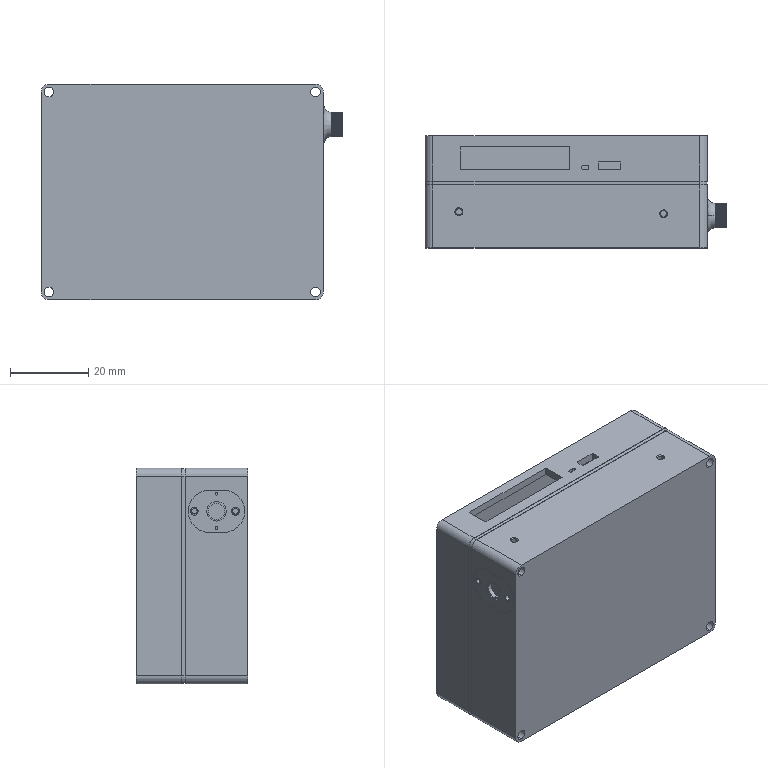Part | SolidWorks | features BaseBody 1 | 1 solid | 633 faces | box 77 x 28.5 x 55 mm | volume 24995 mm3 | plane 457 | cylinder 170 | cone 4 | spline 2 | commonest cylinder face diameters 6.201 x100 4 x12 2 x10 0.4 x8 2.5 x8 0.6 x4